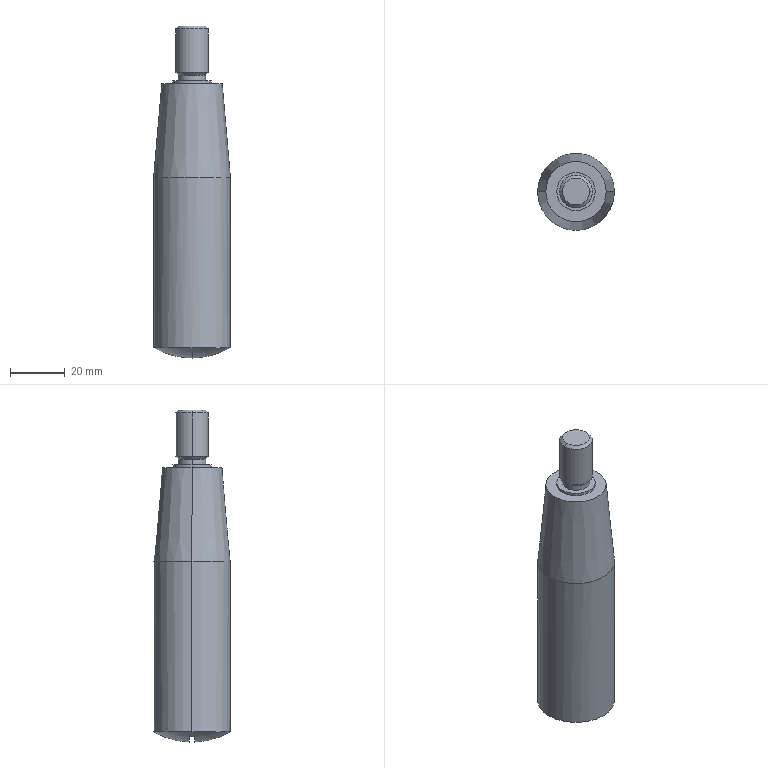Part | SolidWorks | features MBimport 1 | 1 solid | 23 faces | box 28 x 28 x 120.982 mm | volume 58497 mm3 | cylinder 8 | plane 7 | cone 6 | sphere 2 | commonest cylinder face diameters 10 x2 12 x2 14 x2 28 x2
STEP:
#1=CARTESIAN_POINT('',(-14.,0.,-96.249));
#2=VERTEX_POINT('',#1);
#3=CARTESIAN_POINT('',(0.,14.,-96.249));
#4=VERTEX_POINT('',#3);
#5=CARTESIAN_POINT('',(0.,0.,-96.249));
#6=DIRECTION('',(0.,0.,-1.));
#7=DIRECTION('',(-1.,0.,0.));
#8=AXIS2_PLACEMENT_3D('',#5,#6,#7);
#9=CIRCLE('',#8,14.);
#10=EDGE_CURVE('',#2,#4,#9,.T.);
#11=ORIENTED_EDGE('',*,*,#10,.T.);
#12=CARTESIAN_POINT('',(0.,1.,-99.982));
#13=VERTEX_POINT('',#12);
#14=CARTESIAN_POINT('',(0.,0.,-72.));
#15=DIRECTION('',(-1.,0.,0.));
#16=DIRECTION('',(0.,-1.,0.));
#17=AXIS2_PLACEMENT_3D('',#14,#15,#16);
#18=CIRCLE('',#17,28.);
#19=EDGE_CURVE('',#4,#13,#18,.T.);
#20=ORIENTED_EDGE('',*,*,#19,.T.);
#21=CARTESIAN_POINT('',(-10.344,1.,-98.));
#22=VERTEX_POINT('',#21);
#23=CARTESIAN_POINT('',(0.,1.,-72.));
#24=DIRECTION('',(0.,-1.,0.));
#25=DIRECTION('',(0.,0.,1.));
#26=AXIS2_PLACEMENT_3D('',#23,#24,#25);
#27=CIRCLE('',#26,27.982);
#28=EDGE_CURVE('',#22,#13,#27,.T.);
#29=ORIENTED_EDGE('',*,*,#28,.F.);
#30=CARTESIAN_POINT('',(-10.344,-1.,-98.));
#31=VERTEX_POINT('',#30);
#32=CARTESIAN_POINT('',(0.,0.,-98.));
#33=DIRECTION('',(0.,0.,1.));
#34=DIRECTION('',(-1.,0.,0.));
#35=AXIS2_PLACEMENT_3D('',#32,#33,#34);
#36=CIRCLE('',#35,10.392);
#37=EDGE_CURVE('',#22,#31,#36,.T.);
#38=ORIENTED_EDGE('',*,*,#37,.T.);
#39=CARTESIAN_POINT('',(0.,-1.,-99.982));
#40=VERTEX_POINT('',#39);
#41=CARTESIAN_POINT('',(0.,-1.,-72.));
#42=DIRECTION('',(0.,-1.,0.));
#43=DIRECTION('',(0.,0.,1.));
#44=AXIS2_PLACEMENT_3D('',#41,#42,#43);
#45=CIRCLE('',#44,27.982);
#46=EDGE_CURVE('',#31,#40,#45,.T.);
#47=ORIENTED_EDGE('',*,*,#46,.T.);
#48=CARTESIAN_POINT('',(0.,-14.,-96.249));
#49=VERTEX_POINT('',#48);
#50=CARTESIAN_POINT('',(0.,0.,-72.));
#51=DIRECTION('',(1.,0.,0.));
#52=DIRECTION('',(0.,0.,-1.));
#53=AXIS2_PLACEMENT_3D('',#50,#51,#52);
#54=CIRCLE('',#53,28.);
#55=EDGE_CURVE('',#49,#40,#54,.T.);
#56=ORIENTED_EDGE('',*,*,#55,.F.);
#57=CARTESIAN_POINT('',(0.,0.,-96.249));
#58=DIRECTION('',(0.,0.,-1.));
#59=DIRECTION('',(-1.,0.,0.));
#60=AXIS2_PLACEMENT_3D('',#57,#58,#59);
#61=CIRCLE('',#60,14.);
#62=EDGE_CURVE('',#49,#2,#61,.T.);
#63=ORIENTED_EDGE('',*,*,#62,.T.);
#64=EDGE_LOOP('',(#11,#20,#29,#38,#47,#56,#63));
#65=FACE_OUTER_BOUND('',#64,.T.);
#66=CARTESIAN_POINT('',(0.,0.,-72.));
#67=DIRECTION('',(-1.,0.,0.));
#68=DIRECTION('',(0.,-1.,0.));
#69=AXIS2_PLACEMENT_3D('',#66,#67,#68);
#70=SPHERICAL_SURFACE('',#69,28.);
#71=ADVANCED_FACE('',(#65),#70,.T.);
#72=CARTESIAN_POINT('',(14.,0.,-96.249));
#73=VERTEX_POINT('',#72);
#74=CARTESIAN_POINT('',(0.,0.,-96.249));
#75=DIRECTION('',(0.,0.,-1.));
#76=DIRECTION('',(-1.,0.,0.));
#77=AXIS2_PLACEMENT_3D('',#74,#75,#76);
#78=CIRCLE('',#77,14.);
#79=EDGE_CURVE('',#73,#49,#78,.T.);
#80=ORIENTED_EDGE('',*,*,#79,.F.);
#81=CARTESIAN_POINT('',(14.,0.,-34.29));
#82=VERTEX_POINT('',#81);
#83=CARTESIAN_POINT('',(14.,0.,-100.));
#84=DIRECTION('',(0.,0.,1.));
#85=VECTOR('',#84,1000.);
#86=LINE('',#83,#85);
#87=EDGE_CURVE('',#73,#82,#86,.T.);
#88=ORIENTED_EDGE('',*,*,#87,.T.);
#89=CARTESIAN_POINT('',(-14.,0.,-34.29));
#90=VERTEX_POINT('',#89);
#91=CARTESIAN_POINT('',(0.,0.,-34.29));
#92=DIRECTION('',(0.,0.,-1.));
#93=DIRECTION('',(-1.,0.,0.));
#94=AXIS2_PLACEMENT_3D('',#91,#92,#93);
#95=CIRCLE('',#94,14.);
#96=EDGE_CURVE('',#82,#90,#95,.T.);
#97=ORIENTED_EDGE('',*,*,#96,.T.);
#98=CARTESIAN_POINT('',(-14.,0.,-100.));
#99=DIRECTION('',(0.,0.,1.));
#100=VECTOR('',#99,1000.);
#101=LINE('',#98,#100);
#102=EDGE_CURVE('',#2,#90,#101,.T.);
#103=ORIENTED_EDGE('',*,*,#102,.F.);
#104=ORIENTED_EDGE('',*,*,#62,.F.);
#105=EDGE_LOOP('',(#80,#88,#97,#103,#104));
#106=FACE_OUTER_BOUND('',#105,.T.);
#107=CARTESIAN_POINT('',(0.,0.,-100.));
#108=DIRECTION('',(0.,0.,1.));
#109=DIRECTION('',(-1.,0.,0.));
#110=AXIS2_PLACEMENT_3D('',#107,#108,#109);
#111=CYLINDRICAL_SURFACE('',#110,14.);
#112=ADVANCED_FACE('',(#106),#111,.T.);
#113=CARTESIAN_POINT('',(-11.,0.,0.));
#114=VERTEX_POINT('',#113);
#115=CARTESIAN_POINT('',(11.,0.,0.));
#116=VERTEX_POINT('',#115);
#117=CARTESIAN_POINT('',(0.,0.,0.));
#118=DIRECTION('',(0.,0.,-1.));
#119=DIRECTION('',(-1.,0.,0.));
#120=AXIS2_PLACEMENT_3D('',#117,#118,#119);
#121=CIRCLE('',#120,11.);
#122=EDGE_CURVE('',#114,#116,#121,.T.);
#123=ORIENTED_EDGE('',*,*,#122,.T.);
#124=CARTESIAN_POINT('',(11.,0.,0.));
#125=DIRECTION('',(0.08716,0.,-0.9962));
#126=VECTOR('',#125,1000.);
#127=LINE('',#124,#126);
#128=EDGE_CURVE('',#116,#82,#127,.T.);
#129=ORIENTED_EDGE('',*,*,#128,.T.);
#130=CARTESIAN_POINT('',(0.,0.,-34.29));
#131=DIRECTION('',(0.,0.,-1.));
#132=DIRECTION('',(-1.,0.,0.));
#133=AXIS2_PLACEMENT_3D('',#130,#131,#132);
#134=CIRCLE('',#133,14.);
#135=EDGE_CURVE('',#90,#82,#134,.T.);
#136=ORIENTED_EDGE('',*,*,#135,.F.);
#137=CARTESIAN_POINT('',(-11.,0.,0.));
#138=DIRECTION('',(-0.08716,0.,-0.9962));
#139=VECTOR('',#138,1000.);
#140=LINE('',#137,#139);
#141=EDGE_CURVE('',#114,#90,#140,.T.);
#142=ORIENTED_EDGE('',*,*,#141,.F.);
#143=EDGE_LOOP('',(#123,#129,#136,#142));
#144=FACE_OUTER_BOUND('',#143,.T.);
#145=CARTESIAN_POINT('',(0.,0.,0.));
#146=DIRECTION('',(0.,0.,-1.));
#147=DIRECTION('',(-1.,0.,0.));
#148=AXIS2_PLACEMENT_3D('',#145,#146,#147);
#149=CONICAL_SURFACE('',#148,11.,0.08727);
#150=ADVANCED_FACE('',(#144),#149,.T.);
#151=CARTESIAN_POINT('',(7.,0.,0.));
#152=VERTEX_POINT('',#151);
#153=CARTESIAN_POINT('',(-7.,0.,0.));
#154=VERTEX_POINT('',#153);
#155=CARTESIAN_POINT('',(0.,0.,0.));
#156=DIRECTION('',(0.,0.,-1.));
#157=DIRECTION('',(-1.,0.,0.));
#158=AXIS2_PLACEMENT_3D('',#155,#156,#157);
#159=CIRCLE('',#158,7.);
#160=EDGE_CURVE('',#152,#154,#159,.T.);
#161=ORIENTED_EDGE('',*,*,#160,.F.);
#162=CARTESIAN_POINT('',(7.,0.,1.));
#163=VERTEX_POINT('',#162);
#164=CARTESIAN_POINT('',(7.,0.,-100.));
#165=DIRECTION('',(0.,0.,1.));
#166=VECTOR('',#165,1000.);
#167=LINE('',#164,#166);
#168=EDGE_CURVE('',#152,#163,#167,.T.);
#169=ORIENTED_EDGE('',*,*,#168,.T.);
#170=CARTESIAN_POINT('',(-7.,0.,1.));
#171=VERTEX_POINT('',#170);
#172=CARTESIAN_POINT('',(0.,0.,1.));
#173=DIRECTION('',(0.,0.,-1.));
#174=DIRECTION('',(-1.,0.,0.));
#175=AXIS2_PLACEMENT_3D('',#172,#173,#174);
#176=CIRCLE('',#175,7.);
#177=EDGE_CURVE('',#163,#171,#176,.T.);
#178=ORIENTED_EDGE('',*,*,#177,.T.);
#179=CARTESIAN_POINT('',(-7.,0.,-100.));
#180=DIRECTION('',(0.,0.,1.));
#181=VECTOR('',#180,1000.);
#182=LINE('',#179,#181);
#183=EDGE_CURVE('',#154,#171,#182,.T.);
#184=ORIENTED_EDGE('',*,*,#183,.F.);
#185=EDGE_LOOP('',(#161,#169,#178,#184));
#186=FACE_OUTER_BOUND('',#185,.T.);
#187=CARTESIAN_POINT('',(0.,0.,-100.));
#188=DIRECTION('',(0.,0.,1.));
#189=DIRECTION('',(-1.,0.,0.));
#190=AXIS2_PLACEMENT_3D('',#187,#188,#189);
#191=CYLINDRICAL_SURFACE('',#190,7.);
#192=ADVANCED_FACE('',(#186),#191,.T.);
#193=CARTESIAN_POINT('',(5.,0.,1.));
#194=VERTEX_POINT('',#193);
#195=CARTESIAN_POINT('',(-5.,0.,1.));
#196=VERTEX_POINT('',#195);
#197=CARTESIAN_POINT('',(0.,0.,1.));
#198=DIRECTION('',(0.,0.,-1.));
#199=DIRECTION('',(-1.,0.,0.));
#200=AXIS2_PLACEMENT_3D('',#197,#198,#199);
#201=CIRCLE('',#200,5.);
#202=EDGE_CURVE('',#194,#196,#201,.T.);
#203=ORIENTED_EDGE('',*,*,#202,.F.);
#204=CARTESIAN_POINT('',(5.,0.,3.));
#205=VERTEX_POINT('',#204);
#206=CARTESIAN_POINT('',(5.,0.,-100.));
#207=DIRECTION('',(0.,0.,1.));
#208=VECTOR('',#207,1000.);
#209=LINE('',#206,#208);
#210=EDGE_CURVE('',#194,#205,#209,.T.);
#211=ORIENTED_EDGE('',*,*,#210,.T.);
#212=CARTESIAN_POINT('',(-5.,0.,3.));
#213=VERTEX_POINT('',#212);
#214=CARTESIAN_POINT('',(0.,0.,3.));
#215=DIRECTION('',(0.,0.,-1.));
#216=DIRECTION('',(-1.,0.,0.));
#217=AXIS2_PLACEMENT_3D('',#214,#215,#216);
#218=CIRCLE('',#217,5.);
#219=EDGE_CURVE('',#205,#213,#218,.T.);
#220=ORIENTED_EDGE('',*,*,#219,.T.);
#221=CARTESIAN_POINT('',(-5.,0.,-100.));
#222=DIRECTION('',(0.,0.,1.));
#223=VECTOR('',#222,1000.);
#224=LINE('',#221,#223);
#225=EDGE_CURVE('',#196,#213,#224,.T.);
#226=ORIENTED_EDGE('',*,*,#225,.F.);
#227=EDGE_LOOP('',(#203,#211,#220,#226));
#228=FACE_OUTER_BOUND('',#227,.T.);
#229=CARTESIAN_POINT('',(0.,0.,-100.));
#230=DIRECTION('',(0.,0.,1.));
#231=DIRECTION('',(-1.,0.,0.));
#232=AXIS2_PLACEMENT_3D('',#229,#230,#231);
#233=CYLINDRICAL_SURFACE('',#232,5.);
#234=ADVANCED_FACE('',(#228),#233,.T.);
#235=CARTESIAN_POINT('',(-4.927,0.,3.));
#236=VERTEX_POINT('',#235);
#237=CARTESIAN_POINT('',(4.927,0.,3.));
#238=VERTEX_POINT('',#237);
#239=CARTESIAN_POINT('',(0.,0.,3.));
#240=DIRECTION('',(0.,0.,-1.));
#241=DIRECTION('',(-1.,0.,0.));
#242=AXIS2_PLACEMENT_3D('',#239,#240,#241);
#243=CIRCLE('',#242,4.927);
#244=EDGE_CURVE('',#236,#238,#243,.T.);
#245=ORIENTED_EDGE('',*,*,#244,.F.);
#246=CARTESIAN_POINT('',(-6.,0.,4.074));
#247=VERTEX_POINT('',#246);
#248=CARTESIAN_POINT('',(-6.,0.,4.074));
#249=DIRECTION('',(-0.7071,0.,0.7071));
#250=VECTOR('',#249,1000.);
#251=LINE('',#248,#250);
#252=EDGE_CURVE('',#236,#247,#251,.T.);
#253=ORIENTED_EDGE('',*,*,#252,.T.);
#254=CARTESIAN_POINT('',(6.,0.,4.074));
#255=VERTEX_POINT('',#254);
#256=CARTESIAN_POINT('',(0.,0.,4.074));
#257=DIRECTION('',(0.,0.,-1.));
#258=DIRECTION('',(-1.,0.,0.));
#259=AXIS2_PLACEMENT_3D('',#256,#257,#258);
#260=CIRCLE('',#259,6.);
#261=EDGE_CURVE('',#247,#255,#260,.T.);
#262=ORIENTED_EDGE('',*,*,#261,.T.);
#263=CARTESIAN_POINT('',(6.,0.,4.074));
#264=DIRECTION('',(0.7071,0.,0.7071));
#265=VECTOR('',#264,1000.);
#266=LINE('',#263,#265);
#267=EDGE_CURVE('',#238,#255,#266,.T.);
#268=ORIENTED_EDGE('',*,*,#267,.F.);
#269=EDGE_LOOP('',(#245,#253,#262,#268));
#270=FACE_OUTER_BOUND('',#269,.T.);
#271=CARTESIAN_POINT('',(0.,0.,4.074));
#272=DIRECTION('',(0.,0.,1.));
#273=DIRECTION('',(1.,0.,0.));
#274=AXIS2_PLACEMENT_3D('',#271,#272,#273);
#275=CONICAL_SURFACE('',#274,6.,0.7854);
#276=ADVANCED_FACE('',(#270),#275,.T.);
#277=CARTESIAN_POINT('',(0.,0.,4.074));
#278=DIRECTION('',(0.,0.,-1.));
#279=DIRECTION('',(-1.,0.,0.));
#280=AXIS2_PLACEMENT_3D('',#277,#278,#279);
#281=CIRCLE('',#280,6.);
#282=EDGE_CURVE('',#255,#247,#281,.T.);
#283=ORIENTED_EDGE('',*,*,#282,.F.);
#284=CARTESIAN_POINT('',(6.,0.,19.927));
#285=VERTEX_POINT('',#284);
#286=CARTESIAN_POINT('',(6.,0.,-100.));
#287=DIRECTION('',(0.,0.,1.));
#288=VECTOR('',#287,1000.);
#289=LINE('',#286,#288);
#290=EDGE_CURVE('',#255,#285,#289,.T.);
#291=ORIENTED_EDGE('',*,*,#290,.T.);
#292=CARTESIAN_POINT('',(-6.,0.,19.927));
#293=VERTEX_POINT('',#292);
#294=CARTESIAN_POINT('',(0.,0.,19.927));
#295=DIRECTION('',(0.,0.,-1.));
#296=DIRECTION('',(-1.,0.,0.));
#297=AXIS2_PLACEMENT_3D('',#294,#295,#296);
#298=CIRCLE('',#297,6.);
#299=EDGE_CURVE('',#285,#293,#298,.T.);
#300=ORIENTED_EDGE('',*,*,#299,.T.);
#301=CARTESIAN_POINT('',(-6.,0.,-100.));
#302=DIRECTION('',(0.,0.,1.));
#303=VECTOR('',#302,1000.);
#304=LINE('',#301,#303);
#305=EDGE_CURVE('',#247,#293,#304,.T.);
#306=ORIENTED_EDGE('',*,*,#305,.F.);
#307=EDGE_LOOP('',(#283,#291,#300,#306));
#308=FACE_OUTER_BOUND('',#307,.T.);
#309=CARTESIAN_POINT('',(0.,0.,-100.));
#310=DIRECTION('',(0.,0.,1.));
#311=DIRECTION('',(-1.,0.,0.));
#312=AXIS2_PLACEMENT_3D('',#309,#310,#311);
#313=CYLINDRICAL_SURFACE('',#312,6.);
#314=ADVANCED_FACE('',(#308),#313,.T.);
#315=CARTESIAN_POINT('',(-4.927,0.,21.));
#316=VERTEX_POINT('',#315);
#317=CARTESIAN_POINT('',(4.927,0.,21.));
#318=VERTEX_POINT('',#317);
#319=CARTESIAN_POINT('',(0.,0.,21.));
#320=DIRECTION('',(0.,0.,-1.));
#321=DIRECTION('',(-1.,0.,0.));
#322=AXIS2_PLACEMENT_3D('',#319,#320,#321);
#323=CIRCLE('',#322,4.927);
#324=EDGE_CURVE('',#316,#318,#323,.T.);
#325=ORIENTED_EDGE('',*,*,#324,.T.);
#326=CARTESIAN_POINT('',(4.927,0.,21.));
#327=DIRECTION('',(0.7071,0.,-0.7071));
#328=VECTOR('',#327,1000.);
#329=LINE('',#326,#328);
#330=EDGE_CURVE('',#318,#285,#329,.T.);
#331=ORIENTED_EDGE('',*,*,#330,.T.);
#332=CARTESIAN_POINT('',(0.,0.,19.927));
#333=DIRECTION('',(0.,0.,-1.));
#334=DIRECTION('',(-1.,0.,0.));
#335=AXIS2_PLACEMENT_3D('',#332,#333,#334);
#336=CIRCLE('',#335,6.);
#337=EDGE_CURVE('',#293,#285,#336,.T.);
#338=ORIENTED_EDGE('',*,*,#337,.F.);
#339=CARTESIAN_POINT('',(-4.927,0.,21.));
#340=DIRECTION('',(-0.7071,0.,-0.7071));
#341=VECTOR('',#340,1000.);
#342=LINE('',#339,#341);
#343=EDGE_CURVE('',#316,#293,#342,.T.);
#344=ORIENTED_EDGE('',*,*,#343,.F.);
#345=EDGE_LOOP('',(#325,#331,#338,#344));
#346=FACE_OUTER_BOUND('',#345,.T.);
#347=CARTESIAN_POINT('',(0.,0.,21.));
#348=DIRECTION('',(0.,0.,-1.));
#349=DIRECTION('',(-1.,0.,0.));
#350=AXIS2_PLACEMENT_3D('',#347,#348,#349);
#351=CONICAL_SURFACE('',#350,4.927,0.7854);
#352=ADVANCED_FACE('',(#346),#351,.T.);
#353=CARTESIAN_POINT('',(10.344,1.,-98.));
#354=VERTEX_POINT('',#353);
#355=CARTESIAN_POINT('',(-28.,1.,-98.));
#356=DIRECTION('',(1.,0.,0.));
#357=VECTOR('',#356,1000.);
#358=LINE('',#355,#357);
#359=EDGE_CURVE('',#22,#354,#358,.T.);
#360=ORIENTED_EDGE('',*,*,#359,.F.);
#361=ORIENTED_EDGE('',*,*,#28,.T.);
#362=CARTESIAN_POINT('',(0.,1.,-72.));
#363=DIRECTION('',(0.,-1.,0.));
#364=DIRECTION('',(0.,0.,1.));
#365=AXIS2_PLACEMENT_3D('',#362,#363,#364);
#366=CIRCLE('',#365,27.982);
#367=EDGE_CURVE('',#13,#354,#366,.T.);
#368=ORIENTED_EDGE('',*,*,#367,.T.);
#369=EDGE_LOOP('',(#360,#361,#368));
#370=FACE_OUTER_BOUND('',#369,.T.);
#371=CARTESIAN_POINT('',(0.,1.,0.));
#372=DIRECTION('',(0.,1.,0.));
#373=DIRECTION('',(1.,0.,0.));
#374=AXIS2_PLACEMENT_3D('',#371,#372,#373);
#375=PLANE('',#374);
#376=ADVANCED_FACE('',(#370),#375,.F.);
#377=CARTESIAN_POINT('',(10.344,-1.,-98.));
#378=VERTEX_POINT('',#377);
#379=CARTESIAN_POINT('',(-28.,-1.,-98.));
#380=DIRECTION('',(1.,0.,0.));
#381=VECTOR('',#380,1000.);
#382=LINE('',#379,#381);
#383=EDGE_CURVE('',#31,#378,#382,.T.);
#384=ORIENTED_EDGE('',*,*,#383,.T.);
#385=CARTESIAN_POINT('',(0.,-1.,-72.));
#386=DIRECTION('',(0.,-1.,0.));
#387=DIRECTION('',(0.,0.,1.));
#388=AXIS2_PLACEMENT_3D('',#385,#386,#387);
#389=CIRCLE('',#388,27.982);
#390=EDGE_CURVE('',#40,#378,#389,.T.);
#391=ORIENTED_EDGE('',*,*,#390,.F.);
#392=ORIENTED_EDGE('',*,*,#46,.F.);
#393=EDGE_LOOP('',(#384,#391,#392));
#394=FACE_OUTER_BOUND('',#393,.T.);
#395=CARTESIAN_POINT('',(0.,-1.,0.));
#396=DIRECTION('',(0.,1.,0.));
#397=DIRECTION('',(1.,0.,0.));
#398=AXIS2_PLACEMENT_3D('',#395,#396,#397);
#399=PLANE('',#398);
#400=ADVANCED_FACE('',(#394),#399,.T.);
#401=ORIENTED_EDGE('',*,*,#383,.F.);
#402=ORIENTED_EDGE('',*,*,#37,.F.);
#403=ORIENTED_EDGE('',*,*,#359,.T.);
#404=CARTESIAN_POINT('',(0.,0.,-98.));
#405=DIRECTION('',(0.,0.,1.));
#406=DIRECTION('',(-1.,0.,0.));
#407=AXIS2_PLACEMENT_3D('',#404,#405,#406);
#408=CIRCLE('',#407,10.392);
#409=EDGE_CURVE('',#378,#354,#408,.T.);
#410=ORIENTED_EDGE('',*,*,#409,.F.);
#411=EDGE_LOOP('',(#401,#402,#403,#410));
#412=FACE_OUTER_BOUND('',#411,.T.);
#413=CARTESIAN_POINT('',(-28.,1.,-98.));
#414=DIRECTION('',(0.,0.,-1.));
#415=DIRECTION('',(0.,-1.,0.));
#416=AXIS2_PLACEMENT_3D('',#413,#414,#415);
#417=PLANE('',#416);
#418=ADVANCED_FACE('',(#412),#417,.T.);
#419=ORIENTED_EDGE('',*,*,#324,.F.);
#420=CARTESIAN_POINT('',(0.,0.,21.));
#421=DIRECTION('',(0.,0.,-1.));
#422=DIRECTION('',(-1.,0.,0.));
#423=AXIS2_PLACEMENT_3D('',#420,#421,#422);
#424=CIRCLE('',#423,4.927);
#425=EDGE_CURVE('',#318,#316,#424,.T.);
#426=ORIENTED_EDGE('',*,*,#425,.F.);
#427=EDGE_LOOP('',(#419,#426));
#428=FACE_OUTER_BOUND('',#427,.T.);
#429=CARTESIAN_POINT('',(0.,0.,21.));
#430=DIRECTION('',(0.,0.,-1.));
#431=DIRECTION('',(0.,-1.,0.));
#432=AXIS2_PLACEMENT_3D('',#429,#430,#431);
#433=PLANE('',#432);
#434=ADVANCED_FACE('',(#428),#433,.F.);
#435=ORIENTED_EDGE('',*,*,#330,.F.);
#436=ORIENTED_EDGE('',*,*,#425,.T.);
#437=ORIENTED_EDGE('',*,*,#343,.T.);
#438=ORIENTED_EDGE('',*,*,#299,.F.);
#439=EDGE_LOOP('',(#435,#436,#437,#438));
#440=FACE_OUTER_BOUND('',#439,.T.);
#441=CARTESIAN_POINT('',(0.,0.,21.));
#442=DIRECTION('',(0.,0.,-1.));
#443=DIRECTION('',(-1.,0.,0.));
#444=AXIS2_PLACEMENT_3D('',#441,#442,#443);
#445=CONICAL_SURFACE('',#444,4.927,0.7854);
#446=ADVANCED_FACE('',(#440),#445,.T.);
#447=ORIENTED_EDGE('',*,*,#290,.F.);
#448=ORIENTED_EDGE('',*,*,#261,.F.);
#449=ORIENTED_EDGE('',*,*,#305,.T.);
#450=ORIENTED_EDGE('',*,*,#337,.T.);
#451=EDGE_LOOP('',(#447,#448,#449,#450));
#452=FACE_OUTER_BOUND('',#451,.T.);
#453=CARTESIAN_POINT('',(0.,0.,-100.));
#454=DIRECTION('',(0.,0.,1.));
#455=DIRECTION('',(-1.,0.,0.));
#456=AXIS2_PLACEMENT_3D('',#453,#454,#455);
#457=CYLINDRICAL_SURFACE('',#456,6.);
#458=ADVANCED_FACE('',(#452),#457,.T.);
#459=ORIENTED_EDGE('',*,*,#252,.F.);
#460=CARTESIAN_POINT('',(0.,0.,3.));
#461=DIRECTION('',(0.,0.,-1.));
#462=DIRECTION('',(-1.,0.,0.));
#463=AXIS2_PLACEMENT_3D('',#460,#461,#462);
#464=CIRCLE('',#463,4.927);
#465=EDGE_CURVE('',#238,#236,#464,.T.);
#466=ORIENTED_EDGE('',*,*,#465,.F.);
#467=ORIENTED_EDGE('',*,*,#267,.T.);
#468=ORIENTED_EDGE('',*,*,#282,.T.);
#469=EDGE_LOOP('',(#459,#466,#467,#468));
#470=FACE_OUTER_BOUND('',#469,.T.);
#471=CARTESIAN_POINT('',(0.,0.,4.074));
#472=DIRECTION('',(0.,0.,1.));
#473=DIRECTION('',(1.,0.,0.));
#474=AXIS2_PLACEMENT_3D('',#471,#472,#473);
#475=CONICAL_SURFACE('',#474,6.,0.7854);
#476=ADVANCED_FACE('',(#470),#475,.T.);
#477=CARTESIAN_POINT('',(0.,0.,3.));
#478=DIRECTION('',(0.,0.,-1.));
#479=DIRECTION('',(-1.,0.,0.));
#480=AXIS2_PLACEMENT_3D('',#477,#478,#479);
#481=CIRCLE('',#480,5.);
#482=EDGE_CURVE('',#213,#205,#481,.T.);
#483=ORIENTED_EDGE('',*,*,#482,.F.);
#484=ORIENTED_EDGE('',*,*,#219,.F.);
#485=EDGE_LOOP('',(#483,#484));
#486=FACE_OUTER_BOUND('',#485,.T.);
#487=ORIENTED_EDGE('',*,*,#465,.T.);
#488=ORIENTED_EDGE('',*,*,#244,.T.);
#489=EDGE_LOOP('',(#487,#488));
#490=FACE_BOUND('',#489,.T.);
#491=CARTESIAN_POINT('',(0.,4.927,3.));
#492=DIRECTION('',(0.,0.,-1.));
#493=DIRECTION('',(0.,-1.,0.));
#494=AXIS2_PLACEMENT_3D('',#491,#492,#493);
#495=PLANE('',#494);
#496=ADVANCED_FACE('',(#486,#490),#495,.F.);
#497=ORIENTED_EDGE('',*,*,#210,.F.);
#498=CARTESIAN_POINT('',(0.,0.,1.));
#499=DIRECTION('',(0.,0.,-1.));
#500=DIRECTION('',(-1.,0.,0.));
#501=AXIS2_PLACEMENT_3D('',#498,#499,#500);
#502=CIRCLE('',#501,5.);
#503=EDGE_CURVE('',#196,#194,#502,.T.);
#504=ORIENTED_EDGE('',*,*,#503,.F.);
#505=ORIENTED_EDGE('',*,*,#225,.T.);
#506=ORIENTED_EDGE('',*,*,#482,.T.);
#507=EDGE_LOOP('',(#497,#504,#505,#506));
#508=FACE_OUTER_BOUND('',#507,.T.);
#509=CARTESIAN_POINT('',(0.,0.,-100.));
#510=DIRECTION('',(0.,0.,1.));
#511=DIRECTION('',(-1.,0.,0.));
#512=AXIS2_PLACEMENT_3D('',#509,#510,#511);
#513=CYLINDRICAL_SURFACE('',#512,5.);
#514=ADVANCED_FACE('',(#508),#513,.T.);
#515=CARTESIAN_POINT('',(0.,0.,1.));
#516=DIRECTION('',(0.,0.,-1.));
#517=DIRECTION('',(-1.,0.,0.));
#518=AXIS2_PLACEMENT_3D('',#515,#516,#517);
#519=CIRCLE('',#518,7.);
#520=EDGE_CURVE('',#171,#163,#519,.T.);
#521=ORIENTED_EDGE('',*,*,#520,.F.);
#522=ORIENTED_EDGE('',*,*,#177,.F.);
#523=EDGE_LOOP('',(#521,#522));
#524=FACE_OUTER_BOUND('',#523,.T.);
#525=ORIENTED_EDGE('',*,*,#503,.T.);
#526=ORIENTED_EDGE('',*,*,#202,.T.);
#527=EDGE_LOOP('',(#525,#526));
#528=FACE_BOUND('',#527,.T.);
#529=CARTESIAN_POINT('',(0.,5.,1.));
#530=DIRECTION('',(0.,0.,-1.));
#531=DIRECTION('',(0.,-1.,0.));
#532=AXIS2_PLACEMENT_3D('',#529,#530,#531);
#533=PLANE('',#532);
#534=ADVANCED_FACE('',(#524,#528),#533,.F.);
#535=ORIENTED_EDGE('',*,*,#168,.F.);
#536=CARTESIAN_POINT('',(0.,0.,0.));
#537=DIRECTION('',(0.,0.,-1.));
#538=DIRECTION('',(-1.,0.,0.));
#539=AXIS2_PLACEMENT_3D('',#536,#537,#538);
#540=CIRCLE('',#539,7.);
#541=EDGE_CURVE('',#154,#152,#540,.T.);
#542=ORIENTED_EDGE('',*,*,#541,.F.);
#543=ORIENTED_EDGE('',*,*,#183,.T.);
#544=ORIENTED_EDGE('',*,*,#520,.T.);
#545=EDGE_LOOP('',(#535,#542,#543,#544));
#546=FACE_OUTER_BOUND('',#545,.T.);
#547=CARTESIAN_POINT('',(0.,0.,-100.));
#548=DIRECTION('',(0.,0.,1.));
#549=DIRECTION('',(-1.,0.,0.));
#550=AXIS2_PLACEMENT_3D('',#547,#548,#549);
#551=CYLINDRICAL_SURFACE('',#550,7.);
#552=ADVANCED_FACE('',(#546),#551,.T.);
#553=ORIENTED_EDGE('',*,*,#122,.F.);
#554=CARTESIAN_POINT('',(0.,0.,0.));
#555=DIRECTION('',(0.,0.,-1.));
#556=DIRECTION('',(-1.,0.,0.));
#557=AXIS2_PLACEMENT_3D('',#554,#555,#556);
#558=CIRCLE('',#557,11.);
#559=EDGE_CURVE('',#116,#114,#558,.T.);
#560=ORIENTED_EDGE('',*,*,#559,.F.);
#561=EDGE_LOOP('',(#553,#560));
#562=FACE_OUTER_BOUND('',#561,.T.);
#563=ORIENTED_EDGE('',*,*,#541,.T.);
#564=ORIENTED_EDGE('',*,*,#160,.T.);
#565=EDGE_LOOP('',(#563,#564));
#566=FACE_BOUND('',#565,.T.);
#567=CARTESIAN_POINT('',(0.,7.,0.));
#568=DIRECTION('',(0.,0.,-1.));
#569=DIRECTION('',(0.,-1.,0.));
#570=AXIS2_PLACEMENT_3D('',#567,#568,#569);
#571=PLANE('',#570);
#572=ADVANCED_FACE('',(#562,#566),#571,.F.);
#573=ORIENTED_EDGE('',*,*,#128,.F.);
#574=ORIENTED_EDGE('',*,*,#559,.T.);
#575=ORIENTED_EDGE('',*,*,#141,.T.);
#576=ORIENTED_EDGE('',*,*,#96,.F.);
#577=EDGE_LOOP('',(#573,#574,#575,#576));
#578=FACE_OUTER_BOUND('',#577,.T.);
#579=CARTESIAN_POINT('',(0.,0.,0.));
#580=DIRECTION('',(0.,0.,-1.));
#581=DIRECTION('',(-1.,0.,0.));
#582=AXIS2_PLACEMENT_3D('',#579,#580,#581);
#583=CONICAL_SURFACE('',#582,11.,0.08727);
#584=ADVANCED_FACE('',(#578),#583,.T.);
#585=ORIENTED_EDGE('',*,*,#87,.F.);
#586=CARTESIAN_POINT('',(0.,0.,-96.249));
#587=DIRECTION('',(0.,0.,-1.));
#588=DIRECTION('',(-1.,0.,0.));
#589=AXIS2_PLACEMENT_3D('',#586,#587,#588);
#590=CIRCLE('',#589,14.);
#591=EDGE_CURVE('',#4,#73,#590,.T.);
#592=ORIENTED_EDGE('',*,*,#591,.F.);
#593=ORIENTED_EDGE('',*,*,#10,.F.);
#594=ORIENTED_EDGE('',*,*,#102,.T.);
#595=ORIENTED_EDGE('',*,*,#135,.T.);
#596=EDGE_LOOP('',(#585,#592,#593,#594,#595));
#597=FACE_OUTER_BOUND('',#596,.T.);
#598=CARTESIAN_POINT('',(0.,0.,-100.));
#599=DIRECTION('',(0.,0.,1.));
#600=DIRECTION('',(-1.,0.,0.));
#601=AXIS2_PLACEMENT_3D('',#598,#599,#600);
#602=CYLINDRICAL_SURFACE('',#601,14.);
#603=ADVANCED_FACE('',(#597),#602,.T.);
#604=ORIENTED_EDGE('',*,*,#19,.F.);
#605=ORIENTED_EDGE('',*,*,#591,.T.);
#606=ORIENTED_EDGE('',*,*,#79,.T.);
#607=ORIENTED_EDGE('',*,*,#55,.T.);
#608=ORIENTED_EDGE('',*,*,#390,.T.);
#609=ORIENTED_EDGE('',*,*,#409,.T.);
#610=ORIENTED_EDGE('',*,*,#367,.F.);
#611=EDGE_LOOP('',(#604,#605,#606,#607,#608,#609,#610));
#612=FACE_OUTER_BOUND('',#611,.T.);
#613=CARTESIAN_POINT('',(0.,0.,-72.));
#614=DIRECTION('',(-1.,0.,0.));
#615=DIRECTION('',(0.,-1.,0.));
#616=AXIS2_PLACEMENT_3D('',#613,#614,#615);
#617=SPHERICAL_SURFACE('',#616,28.);
#618=ADVANCED_FACE('',(#612),#617,.T.);
#619=CLOSED_SHELL('',(#71,#112,#150,#192,#234,#276,#314,#352,#376,#400,#418,#434,#446,#458,#476,#496,#514,#534,#552,#572,#584,#603,#618));
#620=MANIFOLD_SOLID_BREP('',#619);
#621=CARTESIAN_POINT('',(0.,0.,0.));
#622=DIRECTION('',(0.,0.,1.));
#623=DIRECTION('',(1.,0.,0.));
#624=AXIS2_PLACEMENT_3D('',#621,#622,#623);
#625=(LENGTH_UNIT()NAMED_UNIT(*)SI_UNIT(.MILLI.,.METRE.));
#626=UNCERTAINTY_MEASURE_WITH_UNIT(LENGTH_MEASURE(0.00001),#625,'','');
#627=(NAMED_UNIT(*)PLANE_ANGLE_UNIT()SI_UNIT($,.RADIAN.));
#628=(NAMED_UNIT(*)SI_UNIT($,.STERADIAN.)SOLID_ANGLE_UNIT());
#629=(GEOMETRIC_REPRESENTATION_CONTEXT(3)GLOBAL_UNCERTAINTY_ASSIGNED_CONTEXT((#626))GLOBAL_UNIT_ASSIGNED_CONTEXT((#625,#627,#628))REPRESENTATION_CONTEXT('',''));
#630=ADVANCED_BREP_SHAPE_REPRESENTATION('',(#620,#624),#629);